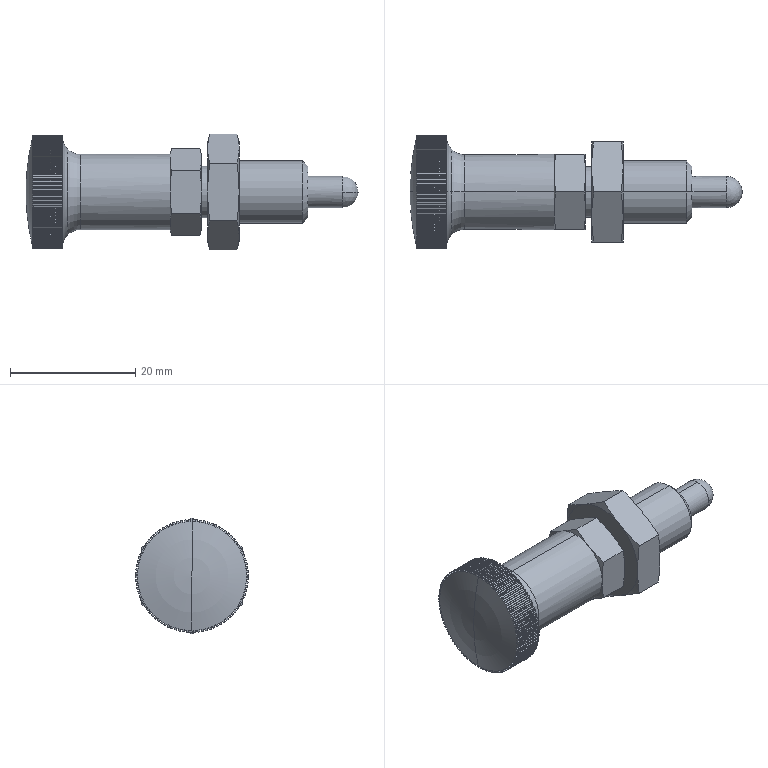Part | NX | features BREP 1 | 1 solid | 646 faces | box 53 x 18 x 18.475 mm | volume 6085 mm3 | cylinder 412 | plane 196 | cone 30 | torus 6 | sphere 2 | commonest cylinder face diameters 0.1 x224 17.4 x90 18 x90 5 x2 8.16 x2 10 x2